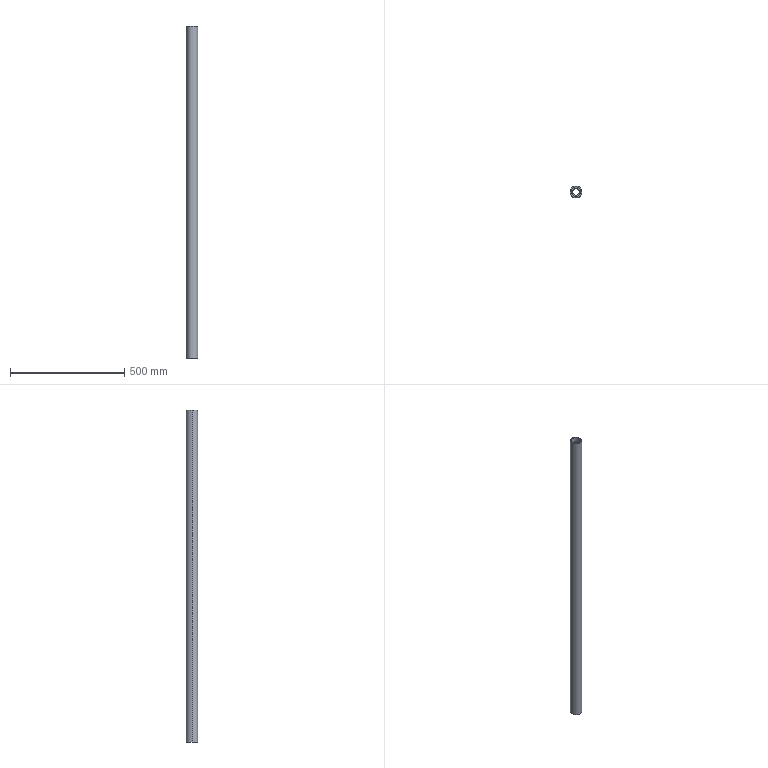Part | STEP file | 1 solid | 12 faces | box 50 x 50 x 1450 mm | volume 1794980 mm3 | cylinder 8 | plane 4 | commonest cylinder face diameters 42 x4 30 x2 50 x2
STEP:
#1=CARTESIAN_POINT('',(0.,0.,0.));
#2=DIRECTION('',(0.,0.,1.));
#3=DIRECTION('',(1.,0.,0.));
#4=AXIS2_PLACEMENT_3D('',#1,#2,#3);
#5=CARTESIAN_POINT('',(-21.,0.,-705.));
#6=VERTEX_POINT('',#5);
#7=CARTESIAN_POINT('',(-21.,0.,-725.));
#8=VERTEX_POINT('',#7);
#9=CARTESIAN_POINT('',(-21.,0.,-705.));
#10=DIRECTION('',(0.,0.,-1.));
#11=VECTOR('',#10,1.);
#12=LINE('',#9,#11);
#13=CARTESIAN_POINT('',(0.,0.,-705.));
#14=DIRECTION('',(0.,0.,-1.));
#15=DIRECTION('',(-1.,0.,0.));
#16=AXIS2_PLACEMENT_3D('',#13,#14,#15);
#17=CYLINDRICAL_SURFACE('',#16,21.);
#18=CARTESIAN_POINT('',(6.283,0.));
#19=DIRECTION('',(0.,1.));
#20=VECTOR('',#19,1.);
#21=LINE('',#18,#20);
#22=(GEOMETRIC_REPRESENTATION_CONTEXT(2)PARAMETRIC_REPRESENTATION_CONTEXT()REPRESENTATION_CONTEXT('',''));
#23=DEFINITIONAL_REPRESENTATION('',(#21),#22);
#24=PCURVE('',#17,#23);
#25=CARTESIAN_POINT('',(0.,0.,-705.));
#26=DIRECTION('',(0.,0.,-1.));
#27=DIRECTION('',(-1.,0.,0.));
#28=AXIS2_PLACEMENT_3D('',#25,#26,#27);
#29=CYLINDRICAL_SURFACE('',#28,21.);
#30=CARTESIAN_POINT('',(0.,0.));
#31=DIRECTION('',(0.,1.));
#32=VECTOR('',#31,1.);
#33=LINE('',#30,#32);
#34=(GEOMETRIC_REPRESENTATION_CONTEXT(2)PARAMETRIC_REPRESENTATION_CONTEXT()REPRESENTATION_CONTEXT('',''));
#35=DEFINITIONAL_REPRESENTATION('',(#33),#34);
#36=PCURVE('',#29,#35);
#37=SURFACE_CURVE('',#12,(#24,#36),.PCURVE_S1.);
#38=EDGE_CURVE('',#6,#8,#37,.T.);
#39=ORIENTED_EDGE('',*,*,#38,.T.);
#40=CARTESIAN_POINT('',(21.,0.,-725.));
#41=VERTEX_POINT('',#40);
#42=CARTESIAN_POINT('',(0.,0.,-725.));
#43=DIRECTION('',(0.,0.,1.));
#44=DIRECTION('',(1.,0.,0.));
#45=AXIS2_PLACEMENT_3D('',#42,#43,#44);
#46=CIRCLE('',#45,21.);
#47=CARTESIAN_POINT('',(9.425,20.));
#48=DIRECTION('',(-1.,0.));
#49=VECTOR('',#48,1.);
#50=LINE('',#47,#49);
#51=(GEOMETRIC_REPRESENTATION_CONTEXT(2)PARAMETRIC_REPRESENTATION_CONTEXT()REPRESENTATION_CONTEXT('',''));
#52=DEFINITIONAL_REPRESENTATION('',(#50),#51);
#53=PCURVE('',#17,#52);
#54=CARTESIAN_POINT('',(0.,0.,-725.));
#55=DIRECTION('',(0.,0.,1.));
#56=DIRECTION('',(1.,0.,0.));
#57=AXIS2_PLACEMENT_3D('',#54,#55,#56);
#58=PLANE('',#57);
#59=CARTESIAN_POINT('',(0.,0.));
#60=DIRECTION('',(1.,0.));
#61=AXIS2_PLACEMENT_2D('',#59,#60);
#62=CIRCLE('',#61,21.);
#63=(GEOMETRIC_REPRESENTATION_CONTEXT(2)PARAMETRIC_REPRESENTATION_CONTEXT()REPRESENTATION_CONTEXT('',''));
#64=DEFINITIONAL_REPRESENTATION('',(#62),#63);
#65=PCURVE('',#58,#64);
#66=SURFACE_CURVE('',#46,(#53,#65),.PCURVE_S1.);
#67=EDGE_CURVE('',#8,#41,#66,.T.);
#68=ORIENTED_EDGE('',*,*,#67,.T.);
#69=CARTESIAN_POINT('',(21.,0.,-705.));
#70=VERTEX_POINT('',#69);
#71=CARTESIAN_POINT('',(21.,0.,-705.));
#72=DIRECTION('',(0.,0.,-1.));
#73=VECTOR('',#72,1.);
#74=LINE('',#71,#73);
#75=CARTESIAN_POINT('',(3.142,0.));
#76=DIRECTION('',(0.,1.));
#77=VECTOR('',#76,1.);
#78=LINE('',#75,#77);
#79=(GEOMETRIC_REPRESENTATION_CONTEXT(2)PARAMETRIC_REPRESENTATION_CONTEXT()REPRESENTATION_CONTEXT('',''));
#80=DEFINITIONAL_REPRESENTATION('',(#78),#79);
#81=PCURVE('',#17,#80);
#82=CARTESIAN_POINT('',(3.142,0.));
#83=DIRECTION('',(0.,1.));
#84=VECTOR('',#83,1.);
#85=LINE('',#82,#84);
#86=(GEOMETRIC_REPRESENTATION_CONTEXT(2)PARAMETRIC_REPRESENTATION_CONTEXT()REPRESENTATION_CONTEXT('',''));
#87=DEFINITIONAL_REPRESENTATION('',(#85),#86);
#88=PCURVE('',#29,#87);
#89=SURFACE_CURVE('',#74,(#81,#88),.PCURVE_S1.);
#90=EDGE_CURVE('',#70,#41,#89,.T.);
#91=ORIENTED_EDGE('',*,*,#90,.F.);
#92=CARTESIAN_POINT('',(0.,0.,-705.));
#93=DIRECTION('',(0.,0.,1.));
#94=DIRECTION('',(1.,0.,0.));
#95=AXIS2_PLACEMENT_3D('',#92,#93,#94);
#96=CIRCLE('',#95,21.);
#97=CARTESIAN_POINT('',(9.425,0.));
#98=DIRECTION('',(-1.,0.));
#99=VECTOR('',#98,1.);
#100=LINE('',#97,#99);
#101=(GEOMETRIC_REPRESENTATION_CONTEXT(2)PARAMETRIC_REPRESENTATION_CONTEXT()REPRESENTATION_CONTEXT('',''));
#102=DEFINITIONAL_REPRESENTATION('',(#100),#101);
#103=PCURVE('',#17,#102);
#104=CARTESIAN_POINT('',(0.,0.,-705.));
#105=DIRECTION('',(0.,0.,-1.));
#106=DIRECTION('',(1.,0.,0.));
#107=AXIS2_PLACEMENT_3D('',#104,#105,#106);
#108=PLANE('',#107);
#109=CARTESIAN_POINT('',(21.,0.));
#110=CARTESIAN_POINT('',(21.,-36.373));
#111=CARTESIAN_POINT('',(-10.5,-18.187));
#112=CARTESIAN_POINT('',(-42.,0.));
#113=CARTESIAN_POINT('',(-10.5,18.187));
#114=CARTESIAN_POINT('',(21.,36.373));
#115=CARTESIAN_POINT('',(21.,0.));
#116=(BOUNDED_CURVE()B_SPLINE_CURVE(2,(#109,#110,#111,#112,#113,#114,#115),.UNSPECIFIED.,.T.,.F.)B_SPLINE_CURVE_WITH_KNOTS((1,2,2,2,2,1),(-2.094,0.,2.094,4.189,6.283,8.378),.UNSPECIFIED.)CURVE()GEOMETRIC_REPRESENTATION_ITEM()RATIONAL_B_SPLINE_CURVE((1.,0.5,1.,0.5,1.,0.5,1.))REPRESENTATION_ITEM(''));
#117=(GEOMETRIC_REPRESENTATION_CONTEXT(2)PARAMETRIC_REPRESENTATION_CONTEXT()REPRESENTATION_CONTEXT('',''));
#118=DEFINITIONAL_REPRESENTATION('',(#116),#117);
#119=PCURVE('',#108,#118);
#120=SURFACE_CURVE('',#96,(#103,#119),.PCURVE_S1.);
#121=EDGE_CURVE('',#6,#70,#120,.T.);
#122=ORIENTED_EDGE('',*,*,#121,.F.);
#123=EDGE_LOOP('',(#39,#68,#91,#122));
#124=FACE_BOUND('',#123,.F.);
#125=ADVANCED_FACE('',(#124),#17,.F.);
#126=CARTESIAN_POINT('',(21.,0.,705.));
#127=VERTEX_POINT('',#126);
#128=CARTESIAN_POINT('',(21.,0.,725.));
#129=VERTEX_POINT('',#128);
#130=CARTESIAN_POINT('',(21.,0.,705.));
#131=DIRECTION('',(0.,0.,1.));
#132=VECTOR('',#131,1.);
#133=LINE('',#130,#132);
#134=CARTESIAN_POINT('',(0.,0.,705.));
#135=DIRECTION('',(0.,0.,1.));
#136=DIRECTION('',(1.,0.,0.));
#137=AXIS2_PLACEMENT_3D('',#134,#135,#136);
#138=CYLINDRICAL_SURFACE('',#137,21.);
#139=CARTESIAN_POINT('',(6.283,0.));
#140=DIRECTION('',(0.,1.));
#141=VECTOR('',#140,1.);
#142=LINE('',#139,#141);
#143=(GEOMETRIC_REPRESENTATION_CONTEXT(2)PARAMETRIC_REPRESENTATION_CONTEXT()REPRESENTATION_CONTEXT('',''));
#144=DEFINITIONAL_REPRESENTATION('',(#142),#143);
#145=PCURVE('',#138,#144);
#146=CARTESIAN_POINT('',(0.,0.,705.));
#147=DIRECTION('',(0.,0.,1.));
#148=DIRECTION('',(1.,0.,0.));
#149=AXIS2_PLACEMENT_3D('',#146,#147,#148);
#150=CYLINDRICAL_SURFACE('',#149,21.);
#151=CARTESIAN_POINT('',(0.,0.));
#152=DIRECTION('',(0.,1.));
#153=VECTOR('',#152,1.);
#154=LINE('',#151,#153);
#155=(GEOMETRIC_REPRESENTATION_CONTEXT(2)PARAMETRIC_REPRESENTATION_CONTEXT()REPRESENTATION_CONTEXT('',''));
#156=DEFINITIONAL_REPRESENTATION('',(#154),#155);
#157=PCURVE('',#150,#156);
#158=SURFACE_CURVE('',#133,(#145,#157),.PCURVE_S1.);
#159=EDGE_CURVE('',#127,#129,#158,.T.);
#160=ORIENTED_EDGE('',*,*,#159,.T.);
#161=CARTESIAN_POINT('',(-21.,0.,725.));
#162=VERTEX_POINT('',#161);
#163=CARTESIAN_POINT('',(0.,0.,725.));
#164=DIRECTION('',(0.,0.,1.));
#165=DIRECTION('',(1.,0.,0.));
#166=AXIS2_PLACEMENT_3D('',#163,#164,#165);
#167=CIRCLE('',#166,21.);
#168=CARTESIAN_POINT('',(0.,20.));
#169=DIRECTION('',(1.,0.));
#170=VECTOR('',#169,1.);
#171=LINE('',#168,#170);
#172=(GEOMETRIC_REPRESENTATION_CONTEXT(2)PARAMETRIC_REPRESENTATION_CONTEXT()REPRESENTATION_CONTEXT('',''));
#173=DEFINITIONAL_REPRESENTATION('',(#171),#172);
#174=PCURVE('',#138,#173);
#175=CARTESIAN_POINT('',(0.,0.,725.));
#176=DIRECTION('',(0.,0.,1.));
#177=DIRECTION('',(1.,0.,0.));
#178=AXIS2_PLACEMENT_3D('',#175,#176,#177);
#179=PLANE('',#178);
#180=CARTESIAN_POINT('',(0.,0.));
#181=DIRECTION('',(1.,0.));
#182=AXIS2_PLACEMENT_2D('',#180,#181);
#183=CIRCLE('',#182,21.);
#184=(GEOMETRIC_REPRESENTATION_CONTEXT(2)PARAMETRIC_REPRESENTATION_CONTEXT()REPRESENTATION_CONTEXT('',''));
#185=DEFINITIONAL_REPRESENTATION('',(#183),#184);
#186=PCURVE('',#179,#185);
#187=SURFACE_CURVE('',#167,(#174,#186),.PCURVE_S1.);
#188=EDGE_CURVE('',#162,#129,#187,.T.);
#189=ORIENTED_EDGE('',*,*,#188,.F.);
#190=CARTESIAN_POINT('',(-21.,0.,705.));
#191=VERTEX_POINT('',#190);
#192=CARTESIAN_POINT('',(-21.,0.,705.));
#193=DIRECTION('',(0.,0.,1.));
#194=VECTOR('',#193,1.);
#195=LINE('',#192,#194);
#196=CARTESIAN_POINT('',(3.142,0.));
#197=DIRECTION('',(0.,1.));
#198=VECTOR('',#197,1.);
#199=LINE('',#196,#198);
#200=(GEOMETRIC_REPRESENTATION_CONTEXT(2)PARAMETRIC_REPRESENTATION_CONTEXT()REPRESENTATION_CONTEXT('',''));
#201=DEFINITIONAL_REPRESENTATION('',(#199),#200);
#202=PCURVE('',#138,#201);
#203=CARTESIAN_POINT('',(3.142,0.));
#204=DIRECTION('',(0.,1.));
#205=VECTOR('',#204,1.);
#206=LINE('',#203,#205);
#207=(GEOMETRIC_REPRESENTATION_CONTEXT(2)PARAMETRIC_REPRESENTATION_CONTEXT()REPRESENTATION_CONTEXT('',''));
#208=DEFINITIONAL_REPRESENTATION('',(#206),#207);
#209=PCURVE('',#150,#208);
#210=SURFACE_CURVE('',#195,(#202,#209),.PCURVE_S1.);
#211=EDGE_CURVE('',#191,#162,#210,.T.);
#212=ORIENTED_EDGE('',*,*,#211,.F.);
#213=CARTESIAN_POINT('',(0.,0.,705.));
#214=DIRECTION('',(0.,0.,1.));
#215=DIRECTION('',(1.,0.,0.));
#216=AXIS2_PLACEMENT_3D('',#213,#214,#215);
#217=CIRCLE('',#216,21.);
#218=CARTESIAN_POINT('',(0.,0.));
#219=DIRECTION('',(1.,0.));
#220=VECTOR('',#219,1.);
#221=LINE('',#218,#220);
#222=(GEOMETRIC_REPRESENTATION_CONTEXT(2)PARAMETRIC_REPRESENTATION_CONTEXT()REPRESENTATION_CONTEXT('',''));
#223=DEFINITIONAL_REPRESENTATION('',(#221),#222);
#224=PCURVE('',#138,#223);
#225=CARTESIAN_POINT('',(0.,0.,705.));
#226=DIRECTION('',(0.,0.,1.));
#227=DIRECTION('',(1.,0.,0.));
#228=AXIS2_PLACEMENT_3D('',#225,#226,#227);
#229=PLANE('',#228);
#230=CARTESIAN_POINT('',(0.,0.));
#231=DIRECTION('',(1.,0.));
#232=AXIS2_PLACEMENT_2D('',#230,#231);
#233=CIRCLE('',#232,21.);
#234=(GEOMETRIC_REPRESENTATION_CONTEXT(2)PARAMETRIC_REPRESENTATION_CONTEXT()REPRESENTATION_CONTEXT('',''));
#235=DEFINITIONAL_REPRESENTATION('',(#233),#234);
#236=PCURVE('',#229,#235);
#237=SURFACE_CURVE('',#217,(#224,#236),.PCURVE_S1.);
#238=EDGE_CURVE('',#191,#127,#237,.T.);
#239=ORIENTED_EDGE('',*,*,#238,.T.);
#240=EDGE_LOOP('',(#160,#189,#212,#239));
#241=FACE_BOUND('',#240,.F.);
#242=ADVANCED_FACE('',(#241),#138,.F.);
#243=CARTESIAN_POINT('',(25.,0.,725.));
#244=VERTEX_POINT('',#243);
#245=CARTESIAN_POINT('',(-25.,0.,725.));
#246=VERTEX_POINT('',#245);
#247=CARTESIAN_POINT('',(0.,0.,725.));
#248=DIRECTION('',(0.,0.,1.));
#249=DIRECTION('',(1.,0.,0.));
#250=AXIS2_PLACEMENT_3D('',#247,#248,#249);
#251=CIRCLE('',#250,25.);
#252=CARTESIAN_POINT('',(0.,0.,725.));
#253=DIRECTION('',(0.,0.,-1.));
#254=DIRECTION('',(-1.,0.,0.));
#255=AXIS2_PLACEMENT_3D('',#252,#253,#254);
#256=CYLINDRICAL_SURFACE('',#255,25.);
#257=CARTESIAN_POINT('',(3.142,0.));
#258=DIRECTION('',(-1.,0.));
#259=VECTOR('',#258,1.);
#260=LINE('',#257,#259);
#261=(GEOMETRIC_REPRESENTATION_CONTEXT(2)PARAMETRIC_REPRESENTATION_CONTEXT()REPRESENTATION_CONTEXT('',''));
#262=DEFINITIONAL_REPRESENTATION('',(#260),#261);
#263=PCURVE('',#256,#262);
#264=CARTESIAN_POINT('',(0.,0.));
#265=DIRECTION('',(1.,0.));
#266=AXIS2_PLACEMENT_2D('',#264,#265);
#267=CIRCLE('',#266,25.);
#268=(GEOMETRIC_REPRESENTATION_CONTEXT(2)PARAMETRIC_REPRESENTATION_CONTEXT()REPRESENTATION_CONTEXT('',''));
#269=DEFINITIONAL_REPRESENTATION('',(#267),#268);
#270=PCURVE('',#179,#269);
#271=SURFACE_CURVE('',#251,(#263,#270),.PCURVE_S1.);
#272=EDGE_CURVE('',#244,#246,#271,.T.);
#273=ORIENTED_EDGE('',*,*,#272,.F.);
#274=CARTESIAN_POINT('',(25.,0.,-725.));
#275=VERTEX_POINT('',#274);
#276=CARTESIAN_POINT('',(25.,0.,725.));
#277=DIRECTION('',(0.,0.,-1.));
#278=VECTOR('',#277,1.);
#279=LINE('',#276,#278);
#280=CARTESIAN_POINT('',(3.142,0.));
#281=DIRECTION('',(0.,1.));
#282=VECTOR('',#281,1.);
#283=LINE('',#280,#282);
#284=(GEOMETRIC_REPRESENTATION_CONTEXT(2)PARAMETRIC_REPRESENTATION_CONTEXT()REPRESENTATION_CONTEXT('',''));
#285=DEFINITIONAL_REPRESENTATION('',(#283),#284);
#286=PCURVE('',#256,#285);
#287=CARTESIAN_POINT('',(0.,0.,725.));
#288=DIRECTION('',(0.,0.,-1.));
#289=DIRECTION('',(-1.,0.,0.));
#290=AXIS2_PLACEMENT_3D('',#287,#288,#289);
#291=CYLINDRICAL_SURFACE('',#290,25.);
#292=CARTESIAN_POINT('',(3.142,0.));
#293=DIRECTION('',(0.,1.));
#294=VECTOR('',#293,1.);
#295=LINE('',#292,#294);
#296=(GEOMETRIC_REPRESENTATION_CONTEXT(2)PARAMETRIC_REPRESENTATION_CONTEXT()REPRESENTATION_CONTEXT('',''));
#297=DEFINITIONAL_REPRESENTATION('',(#295),#296);
#298=PCURVE('',#291,#297);
#299=SURFACE_CURVE('',#279,(#286,#298),.PCURVE_S1.);
#300=EDGE_CURVE('',#244,#275,#299,.T.);
#301=ORIENTED_EDGE('',*,*,#300,.T.);
#302=CARTESIAN_POINT('',(-25.,0.,-725.));
#303=VERTEX_POINT('',#302);
#304=CARTESIAN_POINT('',(0.,0.,-725.));
#305=DIRECTION('',(0.,0.,1.));
#306=DIRECTION('',(1.,0.,0.));
#307=AXIS2_PLACEMENT_3D('',#304,#305,#306);
#308=CIRCLE('',#307,25.);
#309=CARTESIAN_POINT('',(3.142,1450.));
#310=DIRECTION('',(-1.,0.));
#311=VECTOR('',#310,1.);
#312=LINE('',#309,#311);
#313=(GEOMETRIC_REPRESENTATION_CONTEXT(2)PARAMETRIC_REPRESENTATION_CONTEXT()REPRESENTATION_CONTEXT('',''));
#314=DEFINITIONAL_REPRESENTATION('',(#312),#313);
#315=PCURVE('',#256,#314);
#316=CARTESIAN_POINT('',(0.,0.));
#317=DIRECTION('',(1.,0.));
#318=AXIS2_PLACEMENT_2D('',#316,#317);
#319=CIRCLE('',#318,25.);
#320=(GEOMETRIC_REPRESENTATION_CONTEXT(2)PARAMETRIC_REPRESENTATION_CONTEXT()REPRESENTATION_CONTEXT('',''));
#321=DEFINITIONAL_REPRESENTATION('',(#319),#320);
#322=PCURVE('',#58,#321);
#323=SURFACE_CURVE('',#308,(#315,#322),.PCURVE_S1.);
#324=EDGE_CURVE('',#275,#303,#323,.T.);
#325=ORIENTED_EDGE('',*,*,#324,.T.);
#326=CARTESIAN_POINT('',(-25.,0.,725.));
#327=DIRECTION('',(0.,0.,-1.));
#328=VECTOR('',#327,1.);
#329=LINE('',#326,#328);
#330=CARTESIAN_POINT('',(0.,0.));
#331=DIRECTION('',(0.,1.));
#332=VECTOR('',#331,1.);
#333=LINE('',#330,#332);
#334=(GEOMETRIC_REPRESENTATION_CONTEXT(2)PARAMETRIC_REPRESENTATION_CONTEXT()REPRESENTATION_CONTEXT('',''));
#335=DEFINITIONAL_REPRESENTATION('',(#333),#334);
#336=PCURVE('',#256,#335);
#337=CARTESIAN_POINT('',(6.283,0.));
#338=DIRECTION('',(0.,1.));
#339=VECTOR('',#338,1.);
#340=LINE('',#337,#339);
#341=(GEOMETRIC_REPRESENTATION_CONTEXT(2)PARAMETRIC_REPRESENTATION_CONTEXT()REPRESENTATION_CONTEXT('',''));
#342=DEFINITIONAL_REPRESENTATION('',(#340),#341);
#343=PCURVE('',#291,#342);
#344=SURFACE_CURVE('',#329,(#336,#343),.PCURVE_S1.);
#345=EDGE_CURVE('',#246,#303,#344,.T.);
#346=ORIENTED_EDGE('',*,*,#345,.F.);
#347=EDGE_LOOP('',(#273,#301,#325,#346));
#348=FACE_BOUND('',#347,.T.);
#349=ADVANCED_FACE('',(#348),#256,.T.);
#350=CARTESIAN_POINT('',(-15.,0.,705.));
#351=VERTEX_POINT('',#350);
#352=CARTESIAN_POINT('',(-15.,0.,-705.));
#353=VERTEX_POINT('',#352);
#354=CARTESIAN_POINT('',(-15.,0.,725.));
#355=DIRECTION('',(0.,0.,-1.));
#356=VECTOR('',#355,1.);
#357=LINE('',#354,#356);
#358=CARTESIAN_POINT('',(0.,0.,725.));
#359=DIRECTION('',(0.,0.,-1.));
#360=DIRECTION('',(-1.,0.,0.));
#361=AXIS2_PLACEMENT_3D('',#358,#359,#360);
#362=CYLINDRICAL_SURFACE('',#361,15.);
#363=CARTESIAN_POINT('',(6.283,0.));
#364=DIRECTION('',(0.,1.));
#365=VECTOR('',#364,1.);
#366=LINE('',#363,#365);
#367=(GEOMETRIC_REPRESENTATION_CONTEXT(2)PARAMETRIC_REPRESENTATION_CONTEXT()REPRESENTATION_CONTEXT('',''));
#368=DEFINITIONAL_REPRESENTATION('',(#366),#367);
#369=PCURVE('',#362,#368);
#370=CARTESIAN_POINT('',(0.,0.,725.));
#371=DIRECTION('',(0.,0.,-1.));
#372=DIRECTION('',(-1.,0.,0.));
#373=AXIS2_PLACEMENT_3D('',#370,#371,#372);
#374=CYLINDRICAL_SURFACE('',#373,15.);
#375=CARTESIAN_POINT('',(0.,0.));
#376=DIRECTION('',(0.,1.));
#377=VECTOR('',#376,1.);
#378=LINE('',#375,#377);
#379=(GEOMETRIC_REPRESENTATION_CONTEXT(2)PARAMETRIC_REPRESENTATION_CONTEXT()REPRESENTATION_CONTEXT('',''));
#380=DEFINITIONAL_REPRESENTATION('',(#378),#379);
#381=PCURVE('',#374,#380);
#382=SURFACE_CURVE('',#357,(#369,#381),.PCURVE_S1.);
#383=EDGE_CURVE('',#351,#353,#382,.T.);
#384=ORIENTED_EDGE('',*,*,#383,.T.);
#385=CARTESIAN_POINT('',(15.,0.,-705.));
#386=VERTEX_POINT('',#385);
#387=CARTESIAN_POINT('',(0.,0.,-705.));
#388=DIRECTION('',(0.,0.,-1.));
#389=DIRECTION('',(-1.,0.,0.));
#390=AXIS2_PLACEMENT_3D('',#387,#388,#389);
#391=CIRCLE('',#390,15.);
#392=CARTESIAN_POINT('',(0.,1430.));
#393=DIRECTION('',(1.,0.));
#394=VECTOR('',#393,1.);
#395=LINE('',#392,#394);
#396=(GEOMETRIC_REPRESENTATION_CONTEXT(2)PARAMETRIC_REPRESENTATION_CONTEXT()REPRESENTATION_CONTEXT('',''));
#397=DEFINITIONAL_REPRESENTATION('',(#395),#396);
#398=PCURVE('',#362,#397);
#399=CARTESIAN_POINT('',(0.,0.));
#400=DIRECTION('',(-1.,0.));
#401=AXIS2_PLACEMENT_2D('',#399,#400);
#402=CIRCLE('',#401,15.);
#403=(GEOMETRIC_REPRESENTATION_CONTEXT(2)PARAMETRIC_REPRESENTATION_CONTEXT()REPRESENTATION_CONTEXT('',''));
#404=DEFINITIONAL_REPRESENTATION('',(#402),#403);
#405=PCURVE('',#108,#404);
#406=SURFACE_CURVE('',#391,(#398,#405),.PCURVE_S1.);
#407=EDGE_CURVE('',#386,#353,#406,.T.);
#408=ORIENTED_EDGE('',*,*,#407,.F.);
#409=CARTESIAN_POINT('',(15.,0.,705.));
#410=VERTEX_POINT('',#409);
#411=CARTESIAN_POINT('',(15.,0.,725.));
#412=DIRECTION('',(0.,0.,-1.));
#413=VECTOR('',#412,1.);
#414=LINE('',#411,#413);
#415=CARTESIAN_POINT('',(3.142,0.));
#416=DIRECTION('',(0.,1.));
#417=VECTOR('',#416,1.);
#418=LINE('',#415,#417);
#419=(GEOMETRIC_REPRESENTATION_CONTEXT(2)PARAMETRIC_REPRESENTATION_CONTEXT()REPRESENTATION_CONTEXT('',''));
#420=DEFINITIONAL_REPRESENTATION('',(#418),#419);
#421=PCURVE('',#362,#420);
#422=CARTESIAN_POINT('',(3.142,0.));
#423=DIRECTION('',(0.,1.));
#424=VECTOR('',#423,1.);
#425=LINE('',#422,#424);
#426=(GEOMETRIC_REPRESENTATION_CONTEXT(2)PARAMETRIC_REPRESENTATION_CONTEXT()REPRESENTATION_CONTEXT('',''));
#427=DEFINITIONAL_REPRESENTATION('',(#425),#426);
#428=PCURVE('',#374,#427);
#429=SURFACE_CURVE('',#414,(#421,#428),.PCURVE_S1.);
#430=EDGE_CURVE('',#410,#386,#429,.T.);
#431=ORIENTED_EDGE('',*,*,#430,.F.);
#432=CARTESIAN_POINT('',(0.,0.,705.));
#433=DIRECTION('',(0.,0.,1.));
#434=DIRECTION('',(1.,0.,0.));
#435=AXIS2_PLACEMENT_3D('',#432,#433,#434);
#436=CIRCLE('',#435,15.);
#437=CARTESIAN_POINT('',(9.425,20.));
#438=DIRECTION('',(-1.,0.));
#439=VECTOR('',#438,1.);
#440=LINE('',#437,#439);
#441=(GEOMETRIC_REPRESENTATION_CONTEXT(2)PARAMETRIC_REPRESENTATION_CONTEXT()REPRESENTATION_CONTEXT('',''));
#442=DEFINITIONAL_REPRESENTATION('',(#440),#441);
#443=PCURVE('',#362,#442);
#444=CARTESIAN_POINT('',(0.,0.));
#445=DIRECTION('',(1.,0.));
#446=AXIS2_PLACEMENT_2D('',#444,#445);
#447=CIRCLE('',#446,15.);
#448=(GEOMETRIC_REPRESENTATION_CONTEXT(2)PARAMETRIC_REPRESENTATION_CONTEXT()REPRESENTATION_CONTEXT('',''));
#449=DEFINITIONAL_REPRESENTATION('',(#447),#448);
#450=PCURVE('',#229,#449);
#451=SURFACE_CURVE('',#436,(#443,#450),.PCURVE_S1.);
#452=EDGE_CURVE('',#351,#410,#451,.T.);
#453=ORIENTED_EDGE('',*,*,#452,.F.);
#454=EDGE_LOOP('',(#384,#408,#431,#453));
#455=FACE_BOUND('',#454,.F.);
#456=ADVANCED_FACE('',(#455),#362,.F.);
#457=CARTESIAN_POINT('',(0.,0.,-705.));
#458=DIRECTION('',(0.,0.,-1.));
#459=DIRECTION('',(-1.,0.,0.));
#460=AXIS2_PLACEMENT_3D('',#457,#458,#459);
#461=CIRCLE('',#460,15.);
#462=CARTESIAN_POINT('',(0.,1430.));
#463=DIRECTION('',(1.,0.));
#464=VECTOR('',#463,1.);
#465=LINE('',#462,#464);
#466=(GEOMETRIC_REPRESENTATION_CONTEXT(2)PARAMETRIC_REPRESENTATION_CONTEXT()REPRESENTATION_CONTEXT('',''));
#467=DEFINITIONAL_REPRESENTATION('',(#465),#466);
#468=PCURVE('',#374,#467);
#469=CARTESIAN_POINT('',(0.,0.));
#470=DIRECTION('',(-1.,0.));
#471=AXIS2_PLACEMENT_2D('',#469,#470);
#472=CIRCLE('',#471,15.);
#473=(GEOMETRIC_REPRESENTATION_CONTEXT(2)PARAMETRIC_REPRESENTATION_CONTEXT()REPRESENTATION_CONTEXT('',''));
#474=DEFINITIONAL_REPRESENTATION('',(#472),#473);
#475=PCURVE('',#108,#474);
#476=SURFACE_CURVE('',#461,(#468,#475),.PCURVE_S1.);
#477=EDGE_CURVE('',#353,#386,#476,.T.);
#478=ORIENTED_EDGE('',*,*,#477,.F.);
#479=ORIENTED_EDGE('',*,*,#383,.F.);
#480=CARTESIAN_POINT('',(0.,0.,705.));
#481=DIRECTION('',(0.,0.,1.));
#482=DIRECTION('',(1.,0.,0.));
#483=AXIS2_PLACEMENT_3D('',#480,#481,#482);
#484=CIRCLE('',#483,15.);
#485=CARTESIAN_POINT('',(3.142,20.));
#486=DIRECTION('',(-1.,0.));
#487=VECTOR('',#486,1.);
#488=LINE('',#485,#487);
#489=(GEOMETRIC_REPRESENTATION_CONTEXT(2)PARAMETRIC_REPRESENTATION_CONTEXT()REPRESENTATION_CONTEXT('',''));
#490=DEFINITIONAL_REPRESENTATION('',(#488),#489);
#491=PCURVE('',#374,#490);
#492=CARTESIAN_POINT('',(0.,0.));
#493=DIRECTION('',(1.,0.));
#494=AXIS2_PLACEMENT_2D('',#492,#493);
#495=CIRCLE('',#494,15.);
#496=(GEOMETRIC_REPRESENTATION_CONTEXT(2)PARAMETRIC_REPRESENTATION_CONTEXT()REPRESENTATION_CONTEXT('',''));
#497=DEFINITIONAL_REPRESENTATION('',(#495),#496);
#498=PCURVE('',#229,#497);
#499=SURFACE_CURVE('',#484,(#491,#498),.PCURVE_S1.);
#500=EDGE_CURVE('',#410,#351,#499,.T.);
#501=ORIENTED_EDGE('',*,*,#500,.F.);
#502=ORIENTED_EDGE('',*,*,#430,.T.);
#503=EDGE_LOOP('',(#478,#479,#501,#502));
#504=FACE_BOUND('',#503,.F.);
#505=ADVANCED_FACE('',(#504),#374,.F.);
#506=ORIENTED_EDGE('',*,*,#300,.F.);
#507=CARTESIAN_POINT('',(0.,0.,725.));
#508=DIRECTION('',(0.,0.,1.));
#509=DIRECTION('',(1.,0.,0.));
#510=AXIS2_PLACEMENT_3D('',#507,#508,#509);
#511=CIRCLE('',#510,25.);
#512=CARTESIAN_POINT('',(9.425,0.));
#513=DIRECTION('',(-1.,0.));
#514=VECTOR('',#513,1.);
#515=LINE('',#512,#514);
#516=(GEOMETRIC_REPRESENTATION_CONTEXT(2)PARAMETRIC_REPRESENTATION_CONTEXT()REPRESENTATION_CONTEXT('',''));
#517=DEFINITIONAL_REPRESENTATION('',(#515),#516);
#518=PCURVE('',#291,#517);
#519=CARTESIAN_POINT('',(0.,0.));
#520=DIRECTION('',(1.,0.));
#521=AXIS2_PLACEMENT_2D('',#519,#520);
#522=CIRCLE('',#521,25.);
#523=(GEOMETRIC_REPRESENTATION_CONTEXT(2)PARAMETRIC_REPRESENTATION_CONTEXT()REPRESENTATION_CONTEXT('',''));
#524=DEFINITIONAL_REPRESENTATION('',(#522),#523);
#525=PCURVE('',#179,#524);
#526=SURFACE_CURVE('',#511,(#518,#525),.PCURVE_S1.);
#527=EDGE_CURVE('',#246,#244,#526,.T.);
#528=ORIENTED_EDGE('',*,*,#527,.F.);
#529=ORIENTED_EDGE('',*,*,#345,.T.);
#530=CARTESIAN_POINT('',(0.,0.,-725.));
#531=DIRECTION('',(0.,0.,1.));
#532=DIRECTION('',(1.,0.,0.));
#533=AXIS2_PLACEMENT_3D('',#530,#531,#532);
#534=CIRCLE('',#533,25.);
#535=CARTESIAN_POINT('',(9.425,1450.));
#536=DIRECTION('',(-1.,0.));
#537=VECTOR('',#536,1.);
#538=LINE('',#535,#537);
#539=(GEOMETRIC_REPRESENTATION_CONTEXT(2)PARAMETRIC_REPRESENTATION_CONTEXT()REPRESENTATION_CONTEXT('',''));
#540=DEFINITIONAL_REPRESENTATION('',(#538),#539);
#541=PCURVE('',#291,#540);
#542=CARTESIAN_POINT('',(0.,0.));
#543=DIRECTION('',(1.,0.));
#544=AXIS2_PLACEMENT_2D('',#542,#543);
#545=CIRCLE('',#544,25.);
#546=(GEOMETRIC_REPRESENTATION_CONTEXT(2)PARAMETRIC_REPRESENTATION_CONTEXT()REPRESENTATION_CONTEXT('',''));
#547=DEFINITIONAL_REPRESENTATION('',(#545),#546);
#548=PCURVE('',#58,#547);
#549=SURFACE_CURVE('',#534,(#541,#548),.PCURVE_S1.);
#550=EDGE_CURVE('',#303,#275,#549,.T.);
#551=ORIENTED_EDGE('',*,*,#550,.T.);
#552=EDGE_LOOP('',(#506,#528,#529,#551));
#553=FACE_BOUND('',#552,.T.);
#554=ADVANCED_FACE('',(#553),#291,.T.);
#555=CARTESIAN_POINT('',(0.,0.,725.));
#556=DIRECTION('',(0.,0.,1.));
#557=DIRECTION('',(1.,0.,0.));
#558=AXIS2_PLACEMENT_3D('',#555,#556,#557);
#559=CIRCLE('',#558,21.);
#560=CARTESIAN_POINT('',(0.,0.));
#561=DIRECTION('',(1.,0.));
#562=AXIS2_PLACEMENT_2D('',#560,#561);
#563=CIRCLE('',#562,21.);
#564=(GEOMETRIC_REPRESENTATION_CONTEXT(2)PARAMETRIC_REPRESENTATION_CONTEXT()REPRESENTATION_CONTEXT('',''));
#565=DEFINITIONAL_REPRESENTATION('',(#563),#564);
#566=PCURVE('',#179,#565);
#567=CARTESIAN_POINT('',(0.,20.));
#568=DIRECTION('',(1.,0.));
#569=VECTOR('',#568,1.);
#570=LINE('',#567,#569);
#571=(GEOMETRIC_REPRESENTATION_CONTEXT(2)PARAMETRIC_REPRESENTATION_CONTEXT()REPRESENTATION_CONTEXT('',''));
#572=DEFINITIONAL_REPRESENTATION('',(#570),#571);
#573=PCURVE('',#150,#572);
#574=SURFACE_CURVE('',#559,(#566,#573),.PCURVE_S1.);
#575=EDGE_CURVE('',#129,#162,#574,.T.);
#576=ORIENTED_EDGE('',*,*,#575,.F.);
#577=ORIENTED_EDGE('',*,*,#188,.F.);
#578=EDGE_LOOP('',(#576,#577));
#579=FACE_BOUND('',#578,.T.);
#580=ORIENTED_EDGE('',*,*,#527,.T.);
#581=ORIENTED_EDGE('',*,*,#272,.T.);
#582=EDGE_LOOP('',(#580,#581));
#583=FACE_BOUND('',#582,.T.);
#584=ADVANCED_FACE('',(#579,#583),#179,.T.);
#585=ORIENTED_EDGE('',*,*,#67,.T.);
#586=CARTESIAN_POINT('',(0.,0.,-725.));
#587=DIRECTION('',(0.,0.,1.));
#588=DIRECTION('',(1.,0.,0.));
#589=AXIS2_PLACEMENT_3D('',#586,#587,#588);
#590=CIRCLE('',#589,21.);
#591=CARTESIAN_POINT('',(0.,0.));
#592=DIRECTION('',(1.,0.));
#593=AXIS2_PLACEMENT_2D('',#591,#592);
#594=CIRCLE('',#593,21.);
#595=(GEOMETRIC_REPRESENTATION_CONTEXT(2)PARAMETRIC_REPRESENTATION_CONTEXT()REPRESENTATION_CONTEXT('',''));
#596=DEFINITIONAL_REPRESENTATION('',(#594),#595);
#597=PCURVE('',#58,#596);
#598=CARTESIAN_POINT('',(3.142,20.));
#599=DIRECTION('',(-1.,0.));
#600=VECTOR('',#599,1.);
#601=LINE('',#598,#600);
#602=(GEOMETRIC_REPRESENTATION_CONTEXT(2)PARAMETRIC_REPRESENTATION_CONTEXT()REPRESENTATION_CONTEXT('',''));
#603=DEFINITIONAL_REPRESENTATION('',(#601),#602);
#604=PCURVE('',#29,#603);
#605=SURFACE_CURVE('',#590,(#597,#604),.PCURVE_S1.);
#606=EDGE_CURVE('',#41,#8,#605,.T.);
#607=ORIENTED_EDGE('',*,*,#606,.T.);
#608=EDGE_LOOP('',(#585,#607));
#609=FACE_BOUND('',#608,.T.);
#610=ORIENTED_EDGE('',*,*,#550,.F.);
#611=ORIENTED_EDGE('',*,*,#324,.F.);
#612=EDGE_LOOP('',(#610,#611));
#613=FACE_BOUND('',#612,.T.);
#614=ADVANCED_FACE('',(#609,#613),#58,.F.);
#615=ORIENTED_EDGE('',*,*,#575,.F.);
#616=ORIENTED_EDGE('',*,*,#159,.F.);
#617=CARTESIAN_POINT('',(0.,0.,705.));
#618=DIRECTION('',(0.,0.,1.));
#619=DIRECTION('',(1.,0.,0.));
#620=AXIS2_PLACEMENT_3D('',#617,#618,#619);
#621=CIRCLE('',#620,21.);
#622=CARTESIAN_POINT('',(0.,0.));
#623=DIRECTION('',(1.,0.));
#624=VECTOR('',#623,1.);
#625=LINE('',#622,#624);
#626=(GEOMETRIC_REPRESENTATION_CONTEXT(2)PARAMETRIC_REPRESENTATION_CONTEXT()REPRESENTATION_CONTEXT('',''));
#627=DEFINITIONAL_REPRESENTATION('',(#625),#626);
#628=PCURVE('',#150,#627);
#629=CARTESIAN_POINT('',(0.,0.));
#630=DIRECTION('',(1.,0.));
#631=AXIS2_PLACEMENT_2D('',#629,#630);
#632=CIRCLE('',#631,21.);
#633=(GEOMETRIC_REPRESENTATION_CONTEXT(2)PARAMETRIC_REPRESENTATION_CONTEXT()REPRESENTATION_CONTEXT('',''));
#634=DEFINITIONAL_REPRESENTATION('',(#632),#633);
#635=PCURVE('',#229,#634);
#636=SURFACE_CURVE('',#621,(#628,#635),.PCURVE_S1.);
#637=EDGE_CURVE('',#127,#191,#636,.T.);
#638=ORIENTED_EDGE('',*,*,#637,.T.);
#639=ORIENTED_EDGE('',*,*,#211,.T.);
#640=EDGE_LOOP('',(#615,#616,#638,#639));
#641=FACE_BOUND('',#640,.F.);
#642=ADVANCED_FACE('',(#641),#150,.F.);
#643=ORIENTED_EDGE('',*,*,#452,.F.);
#644=ORIENTED_EDGE('',*,*,#500,.F.);
#645=EDGE_LOOP('',(#643,#644));
#646=FACE_BOUND('',#645,.T.);
#647=ORIENTED_EDGE('',*,*,#637,.T.);
#648=ORIENTED_EDGE('',*,*,#238,.T.);
#649=EDGE_LOOP('',(#647,#648));
#650=FACE_BOUND('',#649,.T.);
#651=ADVANCED_FACE('',(#646,#650),#229,.T.);
#652=ORIENTED_EDGE('',*,*,#606,.T.);
#653=ORIENTED_EDGE('',*,*,#38,.F.);
#654=CARTESIAN_POINT('',(0.,0.,-705.));
#655=DIRECTION('',(0.,0.,1.));
#656=DIRECTION('',(1.,0.,0.));
#657=AXIS2_PLACEMENT_3D('',#654,#655,#656);
#658=CIRCLE('',#657,21.);
#659=CARTESIAN_POINT('',(3.142,0.));
#660=DIRECTION('',(-1.,0.));
#661=VECTOR('',#660,1.);
#662=LINE('',#659,#661);
#663=(GEOMETRIC_REPRESENTATION_CONTEXT(2)PARAMETRIC_REPRESENTATION_CONTEXT()REPRESENTATION_CONTEXT('',''));
#664=DEFINITIONAL_REPRESENTATION('',(#662),#663);
#665=PCURVE('',#29,#664);
#666=CARTESIAN_POINT('',(21.,0.));
#667=CARTESIAN_POINT('',(21.,-36.373));
#668=CARTESIAN_POINT('',(-10.5,-18.187));
#669=CARTESIAN_POINT('',(-42.,0.));
#670=CARTESIAN_POINT('',(-10.5,18.187));
#671=CARTESIAN_POINT('',(21.,36.373));
#672=CARTESIAN_POINT('',(21.,0.));
#673=(BOUNDED_CURVE()B_SPLINE_CURVE(2,(#666,#667,#668,#669,#670,#671,#672),.UNSPECIFIED.,.T.,.F.)B_SPLINE_CURVE_WITH_KNOTS((1,2,2,2,2,1),(-2.094,0.,2.094,4.189,6.283,8.378),.UNSPECIFIED.)CURVE()GEOMETRIC_REPRESENTATION_ITEM()RATIONAL_B_SPLINE_CURVE((1.,0.5,1.,0.5,1.,0.5,1.))REPRESENTATION_ITEM(''));
#674=(GEOMETRIC_REPRESENTATION_CONTEXT(2)PARAMETRIC_REPRESENTATION_CONTEXT()REPRESENTATION_CONTEXT('',''));
#675=DEFINITIONAL_REPRESENTATION('',(#673),#674);
#676=PCURVE('',#108,#675);
#677=SURFACE_CURVE('',#658,(#665,#676),.PCURVE_S1.);
#678=EDGE_CURVE('',#70,#6,#677,.T.);
#679=ORIENTED_EDGE('',*,*,#678,.F.);
#680=ORIENTED_EDGE('',*,*,#90,.T.);
#681=EDGE_LOOP('',(#652,#653,#679,#680));
#682=FACE_BOUND('',#681,.F.);
#683=ADVANCED_FACE('',(#682),#29,.F.);
#684=ORIENTED_EDGE('',*,*,#477,.F.);
#685=ORIENTED_EDGE('',*,*,#407,.F.);
#686=EDGE_LOOP('',(#684,#685));
#687=FACE_BOUND('',#686,.T.);
#688=ORIENTED_EDGE('',*,*,#121,.F.);
#689=ORIENTED_EDGE('',*,*,#678,.F.);
#690=EDGE_LOOP('',(#688,#689));
#691=FACE_BOUND('',#690,.T.);
#692=ADVANCED_FACE('',(#687,#691),#108,.T.);
#693=CLOSED_SHELL('',(#125,#242,#349,#456,#505,#554,#584,#614,#642,#651,#683,#692));
#694=MANIFOLD_SOLID_BREP('',#693);
#695=(LENGTH_UNIT()NAMED_UNIT(*)SI_UNIT(.MILLI.,.METRE.));
#696=UNCERTAINTY_MEASURE_WITH_UNIT(LENGTH_MEASURE(0.0000001),#695,'','');
#697=(NAMED_UNIT(*)PLANE_ANGLE_UNIT()SI_UNIT($,.RADIAN.));
#698=(NAMED_UNIT(*)SI_UNIT($,.STERADIAN.)SOLID_ANGLE_UNIT());
#699=(GEOMETRIC_REPRESENTATION_CONTEXT(3)GLOBAL_UNCERTAINTY_ASSIGNED_CONTEXT((#696))GLOBAL_UNIT_ASSIGNED_CONTEXT((#695,#697,#698))REPRESENTATION_CONTEXT('',''));
#700=ADVANCED_BREP_SHAPE_REPRESENTATION('',(#4,#694),#699);